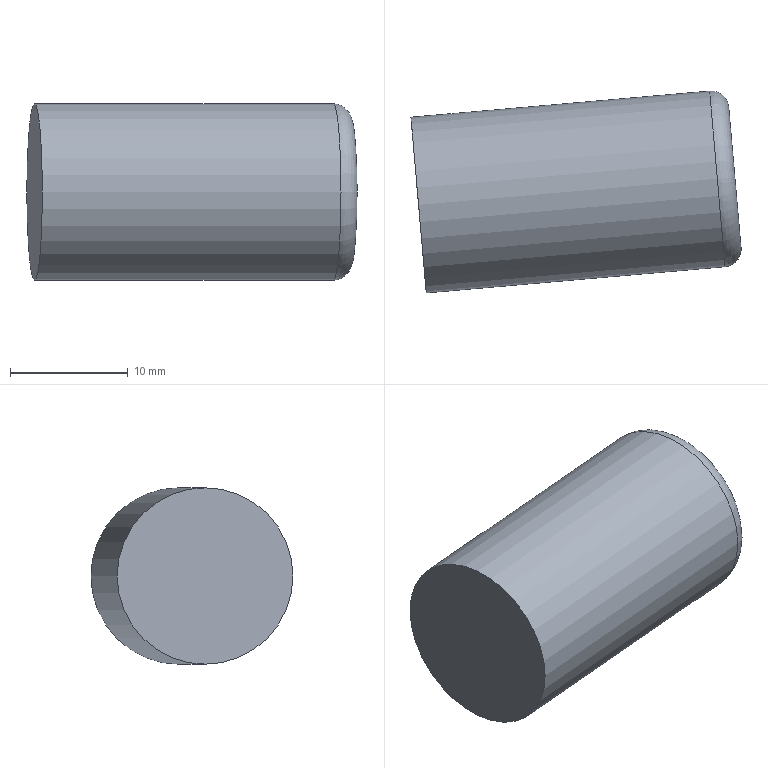Part | NX | features 1 2 | 1 solid | 6 faces | box 28.08 x 17.171 x 15 mm | volume 4719 mm3 | plane 3 | cylinder 2 | torus 1 | commonest cylinder face diameters 2.46 x1 15 x1
STEP:
#1=CARTESIAN_POINT('',(743.149,495.425,-245.));
#2=VERTEX_POINT('',#1);
#3=CARTESIAN_POINT('',(743.042,496.65,-245.));
#4=DIRECTION('',(-0.9962,-0.08716,0.));
#5=DIRECTION('',(0.08716,-0.9962,0.));
#6=AXIS2_PLACEMENT_3D('',#3,#4,#5);
#7=CIRCLE('',#6,1.23);
#8=EDGE_CURVE('',#2,#2,#7,.T.);
#9=ORIENTED_EDGE('',*,*,#8,.F.);
#10=EDGE_LOOP('',(#9));
#11=FACE_BOUND('',#10,.T.);
#12=CARTESIAN_POINT('',(743.042,496.65,-245.));
#13=DIRECTION('',(0.9962,0.08716,0.));
#14=DIRECTION('',(0.,0.,-1.));
#15=AXIS2_PLACEMENT_3D('',#12,#13,#14);
#16=PLANE('',#15);
#17=ADVANCED_FACE('',(#11),#16,.T.);
#18=ORIENTED_EDGE('',*,*,#8,.T.);
#19=EDGE_LOOP('',(#18));
#20=FACE_BOUND('',#19,.T.);
#21=CARTESIAN_POINT('',(749.624,495.991,-245.));
#22=VERTEX_POINT('',#21);
#23=CARTESIAN_POINT('',(749.517,497.217,-245.));
#24=DIRECTION('',(0.9962,0.08716,0.));
#25=DIRECTION('',(0.08716,-0.9962,0.));
#26=AXIS2_PLACEMENT_3D('',#23,#24,#25);
#27=CIRCLE('',#26,1.23);
#28=EDGE_CURVE('',#22,#22,#27,.T.);
#29=ORIENTED_EDGE('',*,*,#28,.T.);
#30=EDGE_LOOP('',(#29));
#31=FACE_BOUND('',#30,.T.);
#32=CARTESIAN_POINT('',(749.517,497.217,-245.));
#33=DIRECTION('',(0.9962,0.08716,0.));
#34=DIRECTION('',(0.,0.,-1.));
#35=AXIS2_PLACEMENT_3D('',#32,#33,#34);
#36=CYLINDRICAL_SURFACE('',#35,1.23);
#37=ADVANCED_FACE('',(#20,#31),#36,.F.);
#38=ORIENTED_EDGE('',*,*,#28,.F.);
#39=EDGE_LOOP('',(#38));
#40=FACE_BOUND('',#39,.T.);
#41=CARTESIAN_POINT('',(750.04,491.24,-245.));
#42=VERTEX_POINT('',#41);
#43=CARTESIAN_POINT('',(749.517,497.217,-245.));
#44=DIRECTION('',(-0.9962,-0.08716,0.));
#45=DIRECTION('',(0.08716,-0.9962,0.));
#46=AXIS2_PLACEMENT_3D('',#43,#44,#45);
#47=CIRCLE('',#46,6.);
#48=EDGE_CURVE('',#42,#42,#47,.T.);
#49=ORIENTED_EDGE('',*,*,#48,.F.);
#50=EDGE_LOOP('',(#49));
#51=FACE_BOUND('',#50,.T.);
#52=CARTESIAN_POINT('',(749.778,494.228,-245.));
#53=DIRECTION('',(0.9962,0.08716,0.));
#54=DIRECTION('',(0.,0.,-1.));
#55=AXIS2_PLACEMENT_3D('',#52,#53,#54);
#56=PLANE('',#55);
#57=ADVANCED_FACE('',(#40,#51),#56,.T.);
#58=CARTESIAN_POINT('',(748.676,489.615,-245.));
#59=VERTEX_POINT('',#58);
#60=CARTESIAN_POINT('',(748.023,497.086,-245.));
#61=DIRECTION('',(-0.9962,-0.08716,0.));
#62=DIRECTION('',(0.08716,-0.9962,0.));
#63=AXIS2_PLACEMENT_3D('',#60,#61,#62);
#64=CIRCLE('',#63,7.5);
#65=EDGE_CURVE('',#59,#59,#64,.T.);
#66=ORIENTED_EDGE('',*,*,#65,.F.);
#67=EDGE_LOOP('',(#66));
#68=FACE_BOUND('',#67,.T.);
#69=ORIENTED_EDGE('',*,*,#48,.T.);
#70=EDGE_LOOP('',(#69));
#71=FACE_BOUND('',#70,.T.);
#72=CARTESIAN_POINT('',(748.023,497.086,-245.));
#73=DIRECTION('',(0.9962,0.08716,0.));
#74=DIRECTION('',(0.,0.,-1.));
#75=AXIS2_PLACEMENT_3D('',#72,#73,#74);
#76=TOROIDAL_SURFACE('',#75,6.,1.5);
#77=ADVANCED_FACE('',(#68,#71),#76,.T.);
#78=CARTESIAN_POINT('',(723.273,487.392,-245.));
#79=VERTEX_POINT('',#78);
#80=CARTESIAN_POINT('',(722.62,494.864,-245.));
#81=DIRECTION('',(0.9962,0.08716,0.));
#82=DIRECTION('',(0.08716,-0.9962,0.));
#83=AXIS2_PLACEMENT_3D('',#80,#81,#82);
#84=CIRCLE('',#83,7.5);
#85=EDGE_CURVE('',#79,#79,#84,.T.);
#86=ORIENTED_EDGE('',*,*,#85,.T.);
#87=EDGE_LOOP('',(#86));
#88=FACE_BOUND('',#87,.T.);
#89=ORIENTED_EDGE('',*,*,#65,.T.);
#90=EDGE_LOOP('',(#89));
#91=FACE_BOUND('',#90,.T.);
#92=CARTESIAN_POINT('',(735.321,495.975,-245.));
#93=DIRECTION('',(-0.9962,-0.08716,0.));
#94=DIRECTION('',(0.,0.,1.));
#95=AXIS2_PLACEMENT_3D('',#92,#93,#94);
#96=CYLINDRICAL_SURFACE('',#95,7.5);
#97=ADVANCED_FACE('',(#88,#91),#96,.T.);
#98=ORIENTED_EDGE('',*,*,#85,.F.);
#99=EDGE_LOOP('',(#98));
#100=FACE_BOUND('',#99,.T.);
#101=CARTESIAN_POINT('',(723.404,485.898,-245.));
#102=DIRECTION('',(0.9962,0.08716,0.));
#103=DIRECTION('',(0.,0.,-1.));
#104=AXIS2_PLACEMENT_3D('',#101,#102,#103);
#105=PLANE('',#104);
#106=ADVANCED_FACE('',(#100),#105,.F.);
#107=CLOSED_SHELL('',(#17,#37,#57,#77,#97,#106));
#108=MANIFOLD_SOLID_BREP('',#107);
#109=(LENGTH_UNIT()NAMED_UNIT(*)SI_UNIT(.MILLI.,.METRE.));
#110=UNCERTAINTY_MEASURE_WITH_UNIT(LENGTH_MEASURE(0.00001),#109,'','');
#111=(NAMED_UNIT(*)PLANE_ANGLE_UNIT()SI_UNIT($,.RADIAN.));
#112=(NAMED_UNIT(*)SI_UNIT($,.STERADIAN.)SOLID_ANGLE_UNIT());
#113=(GEOMETRIC_REPRESENTATION_CONTEXT(3)GLOBAL_UNCERTAINTY_ASSIGNED_CONTEXT((#110))GLOBAL_UNIT_ASSIGNED_CONTEXT((#109,#111,#112))REPRESENTATION_CONTEXT('',''));
#114=ADVANCED_BREP_SHAPE_REPRESENTATION('',(#108),#113);